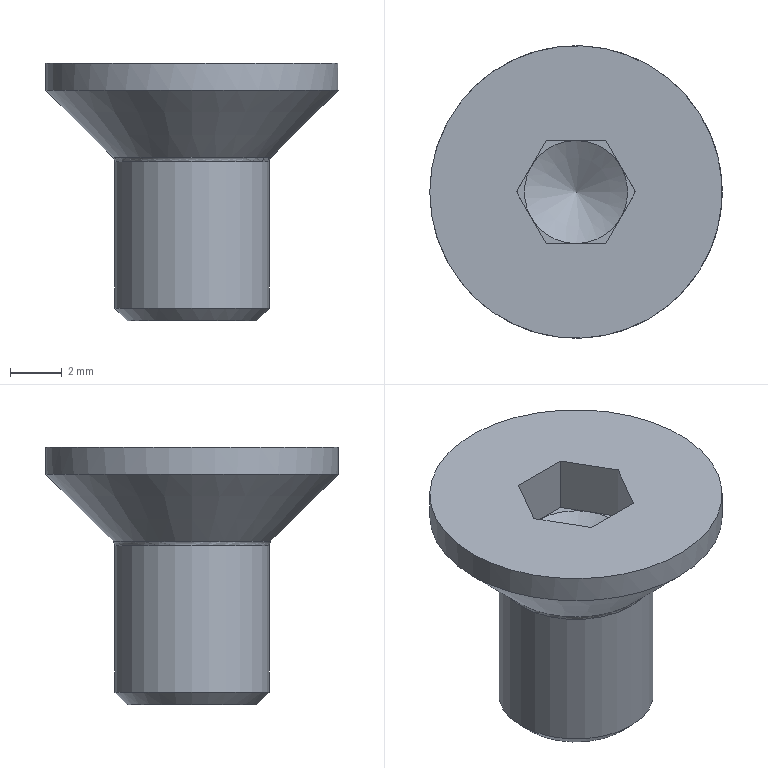Part | STEP file | 冲床-300配套压波_id166_x_t | 1 solid | 20 faces | box 11.34 x 11.34 x 10 mm | volume 408.507 mm3 | plane 14 | cone 3 | cylinder 2 | torus 1 | commonest cylinder face diameters 6 x1 11.34 x1
STEP:
#1=CARTESIAN_POINT('',(1844.33,-85.,217.));
#2=VERTEX_POINT('',#1);
#3=CARTESIAN_POINT('',(1850.,-85.,217.));
#4=DIRECTION('',(0.,0.,-1.));
#5=DIRECTION('',(-1.,0.,0.));
#6=AXIS2_PLACEMENT_3D('',#3,#4,#5);
#7=CIRCLE('',#6,5.67);
#8=EDGE_CURVE('',#2,#2,#7,.T.);
#9=ORIENTED_EDGE('',*,*,#8,.F.);
#10=EDGE_LOOP('',(#9));
#11=FACE_BOUND('',#10,.T.);
#12=CARTESIAN_POINT('',(1847.691,-85.,217.));
#13=VERTEX_POINT('',#12);
#14=CARTESIAN_POINT('',(1848.845,-87.,217.));
#15=VERTEX_POINT('',#14);
#16=CARTESIAN_POINT('',(1847.691,-85.,217.));
#17=DIRECTION('',(0.5,-0.866,0.));
#18=VECTOR('',#17,1.);
#19=LINE('',#16,#18);
#20=EDGE_CURVE('',#13,#15,#19,.T.);
#21=ORIENTED_EDGE('',*,*,#20,.F.);
#22=CARTESIAN_POINT('',(1848.845,-83.,217.));
#23=VERTEX_POINT('',#22);
#24=CARTESIAN_POINT('',(1848.845,-83.,217.));
#25=DIRECTION('',(-0.5,-0.866,0.));
#26=VECTOR('',#25,1.);
#27=LINE('',#24,#26);
#28=EDGE_CURVE('',#23,#13,#27,.T.);
#29=ORIENTED_EDGE('',*,*,#28,.F.);
#30=CARTESIAN_POINT('',(1851.155,-83.,217.));
#31=VERTEX_POINT('',#30);
#32=CARTESIAN_POINT('',(1851.155,-83.,217.));
#33=DIRECTION('',(-1.,0.,0.));
#34=VECTOR('',#33,1.);
#35=LINE('',#32,#34);
#36=EDGE_CURVE('',#31,#23,#35,.T.);
#37=ORIENTED_EDGE('',*,*,#36,.F.);
#38=CARTESIAN_POINT('',(1852.309,-85.,217.));
#39=VERTEX_POINT('',#38);
#40=CARTESIAN_POINT('',(1852.309,-85.,217.));
#41=DIRECTION('',(-0.5,0.866,0.));
#42=VECTOR('',#41,1.);
#43=LINE('',#40,#42);
#44=EDGE_CURVE('',#39,#31,#43,.T.);
#45=ORIENTED_EDGE('',*,*,#44,.F.);
#46=CARTESIAN_POINT('',(1851.155,-87.,217.));
#47=VERTEX_POINT('',#46);
#48=CARTESIAN_POINT('',(1851.155,-87.,217.));
#49=DIRECTION('',(0.5,0.866,0.));
#50=VECTOR('',#49,1.);
#51=LINE('',#48,#50);
#52=EDGE_CURVE('',#47,#39,#51,.T.);
#53=ORIENTED_EDGE('',*,*,#52,.F.);
#54=CARTESIAN_POINT('',(1848.845,-87.,217.));
#55=DIRECTION('',(1.,0.,0.));
#56=VECTOR('',#55,1.);
#57=LINE('',#54,#56);
#58=EDGE_CURVE('',#15,#47,#57,.T.);
#59=ORIENTED_EDGE('',*,*,#58,.F.);
#60=EDGE_LOOP('',(#21,#29,#37,#45,#53,#59));
#61=FACE_BOUND('',#60,.T.);
#62=CARTESIAN_POINT('',(1850.,-85.,217.));
#63=DIRECTION('',(0.,0.,-1.));
#64=DIRECTION('',(-1.,0.,0.));
#65=AXIS2_PLACEMENT_3D('',#62,#63,#64);
#66=PLANE('',#65);
#67=ADVANCED_FACE('',(#11,#61),#66,.F.);
#68=CARTESIAN_POINT('',(1844.33,-85.,215.95));
#69=VERTEX_POINT('',#68);
#70=CARTESIAN_POINT('',(1850.,-85.,215.95));
#71=DIRECTION('',(0.,0.,-1.));
#72=DIRECTION('',(-1.,0.,0.));
#73=AXIS2_PLACEMENT_3D('',#70,#71,#72);
#74=CIRCLE('',#73,5.67);
#75=EDGE_CURVE('',#69,#69,#74,.T.);
#76=ORIENTED_EDGE('',*,*,#75,.F.);
#77=EDGE_LOOP('',(#76));
#78=FACE_BOUND('',#77,.T.);
#79=ORIENTED_EDGE('',*,*,#8,.T.);
#80=EDGE_LOOP('',(#79));
#81=FACE_BOUND('',#80,.T.);
#82=CARTESIAN_POINT('',(1850.,-85.,217.));
#83=DIRECTION('',(0.,0.,-1.));
#84=DIRECTION('',(-1.,0.,0.));
#85=AXIS2_PLACEMENT_3D('',#82,#83,#84);
#86=CYLINDRICAL_SURFACE('',#85,5.67);
#87=ADVANCED_FACE('',(#78,#81),#86,.T.);
#88=CARTESIAN_POINT('',(1853.073,-85.,213.353));
#89=VERTEX_POINT('',#88);
#90=CARTESIAN_POINT('',(1850.,-85.,213.353));
#91=DIRECTION('',(0.,0.,1.));
#92=DIRECTION('',(1.,0.,0.));
#93=AXIS2_PLACEMENT_3D('',#90,#91,#92);
#94=CIRCLE('',#93,3.073);
#95=EDGE_CURVE('',#89,#89,#94,.T.);
#96=ORIENTED_EDGE('',*,*,#95,.T.);
#97=EDGE_LOOP('',(#96));
#98=FACE_BOUND('',#97,.T.);
#99=ORIENTED_EDGE('',*,*,#75,.T.);
#100=EDGE_LOOP('',(#99));
#101=FACE_BOUND('',#100,.T.);
#102=CARTESIAN_POINT('',(1850.,-85.,215.95));
#103=DIRECTION('',(0.,0.,1.));
#104=DIRECTION('',(1.,0.,0.));
#105=AXIS2_PLACEMENT_3D('',#102,#103,#104);
#106=CONICAL_SURFACE('',#105,5.67,45.);
#107=ADVANCED_FACE('',(#98,#101),#106,.T.);
#108=CARTESIAN_POINT('',(1847.,-85.,213.176));
#109=VERTEX_POINT('',#108);
#110=CARTESIAN_POINT('',(1850.,-85.,213.176));
#111=DIRECTION('',(0.,0.,-1.));
#112=DIRECTION('',(-1.,0.,0.));
#113=AXIS2_PLACEMENT_3D('',#110,#111,#112);
#114=CIRCLE('',#113,3.);
#115=EDGE_CURVE('',#109,#109,#114,.T.);
#116=ORIENTED_EDGE('',*,*,#115,.T.);
#117=EDGE_LOOP('',(#116));
#118=FACE_BOUND('',#117,.T.);
#119=CARTESIAN_POINT('',(1853.,-85.,207.5));
#120=VERTEX_POINT('',#119);
#121=CARTESIAN_POINT('',(1850.,-85.,207.5));
#122=DIRECTION('',(0.,0.,1.));
#123=DIRECTION('',(1.,0.,0.));
#124=AXIS2_PLACEMENT_3D('',#121,#122,#123);
#125=CIRCLE('',#124,3.);
#126=EDGE_CURVE('',#120,#120,#125,.T.);
#127=ORIENTED_EDGE('',*,*,#126,.T.);
#128=EDGE_LOOP('',(#127));
#129=FACE_BOUND('',#128,.T.);
#130=CARTESIAN_POINT('',(1850.,-85.,217.));
#131=DIRECTION('',(0.,0.,-1.));
#132=DIRECTION('',(-1.,0.,0.));
#133=AXIS2_PLACEMENT_3D('',#130,#131,#132);
#134=CYLINDRICAL_SURFACE('',#133,3.);
#135=ADVANCED_FACE('',(#118,#129),#134,.T.);
#136=CARTESIAN_POINT('',(1852.5,-85.,207.));
#137=VERTEX_POINT('',#136);
#138=CARTESIAN_POINT('',(1850.,-85.,207.));
#139=DIRECTION('',(0.,0.,-1.));
#140=DIRECTION('',(1.,0.,0.));
#141=AXIS2_PLACEMENT_3D('',#138,#139,#140);
#142=CIRCLE('',#141,2.5);
#143=EDGE_CURVE('',#137,#137,#142,.T.);
#144=ORIENTED_EDGE('',*,*,#143,.T.);
#145=EDGE_LOOP('',(#144));
#146=FACE_OUTER_BOUND('',#145,.T.);
#147=CARTESIAN_POINT('',(1847.,-85.,207.));
#148=DIRECTION('',(0.,0.,1.));
#149=DIRECTION('',(1.,0.,0.));
#150=AXIS2_PLACEMENT_3D('',#147,#148,#149);
#151=PLANE('',#150);
#152=ADVANCED_FACE('',(#146),#151,.F.);
#153=CARTESIAN_POINT('',(1848.268,-86.,214.8));
#154=VERTEX_POINT('',#153);
#155=CARTESIAN_POINT('',(1847.691,-85.,214.8));
#156=VERTEX_POINT('',#155);
#157=CARTESIAN_POINT('',(1847.691,-85.,214.8));
#158=DIRECTION('',(-0.5,0.866,0.));
#159=VECTOR('',#158,1.);
#160=LINE('',#157,#159);
#161=EDGE_CURVE('',#154,#156,#160,.T.);
#162=ORIENTED_EDGE('',*,*,#161,.T.);
#163=CARTESIAN_POINT('',(1847.691,-85.,214.8));
#164=DIRECTION('',(0.,0.,-1.));
#165=VECTOR('',#164,1.);
#166=LINE('',#163,#165);
#167=EDGE_CURVE('',#13,#156,#166,.T.);
#168=ORIENTED_EDGE('',*,*,#167,.F.);
#169=ORIENTED_EDGE('',*,*,#20,.T.);
#170=CARTESIAN_POINT('',(1848.845,-87.,214.8));
#171=VERTEX_POINT('',#170);
#172=CARTESIAN_POINT('',(1848.845,-87.,214.8));
#173=DIRECTION('',(0.,0.,-1.));
#174=VECTOR('',#173,1.);
#175=LINE('',#172,#174);
#176=EDGE_CURVE('',#15,#171,#175,.T.);
#177=ORIENTED_EDGE('',*,*,#176,.T.);
#178=CARTESIAN_POINT('',(1847.691,-85.,214.8));
#179=DIRECTION('',(-0.5,0.866,0.));
#180=VECTOR('',#179,1.);
#181=LINE('',#178,#180);
#182=EDGE_CURVE('',#171,#154,#181,.T.);
#183=ORIENTED_EDGE('',*,*,#182,.T.);
#184=EDGE_LOOP('',(#162,#168,#169,#177,#183));
#185=FACE_OUTER_BOUND('',#184,.T.);
#186=CARTESIAN_POINT('',(1847.691,-85.,214.8));
#187=DIRECTION('',(-0.866,-0.5,0.));
#188=DIRECTION('',(0.5,-0.866,0.));
#189=AXIS2_PLACEMENT_3D('',#186,#187,#188);
#190=PLANE('',#189);
#191=ADVANCED_FACE('',(#185),#190,.F.);
#192=CARTESIAN_POINT('',(1850.,-87.,214.8));
#193=VERTEX_POINT('',#192);
#194=CARTESIAN_POINT('',(1848.845,-87.,214.8));
#195=DIRECTION('',(-1.,0.,0.));
#196=VECTOR('',#195,1.);
#197=LINE('',#194,#196);
#198=EDGE_CURVE('',#193,#171,#197,.T.);
#199=ORIENTED_EDGE('',*,*,#198,.T.);
#200=ORIENTED_EDGE('',*,*,#176,.F.);
#201=ORIENTED_EDGE('',*,*,#58,.T.);
#202=CARTESIAN_POINT('',(1851.155,-87.,214.8));
#203=VERTEX_POINT('',#202);
#204=CARTESIAN_POINT('',(1851.155,-87.,214.8));
#205=DIRECTION('',(0.,0.,-1.));
#206=VECTOR('',#205,1.);
#207=LINE('',#204,#206);
#208=EDGE_CURVE('',#47,#203,#207,.T.);
#209=ORIENTED_EDGE('',*,*,#208,.T.);
#210=CARTESIAN_POINT('',(1848.845,-87.,214.8));
#211=DIRECTION('',(-1.,0.,0.));
#212=VECTOR('',#211,1.);
#213=LINE('',#210,#212);
#214=EDGE_CURVE('',#203,#193,#213,.T.);
#215=ORIENTED_EDGE('',*,*,#214,.T.);
#216=EDGE_LOOP('',(#199,#200,#201,#209,#215));
#217=FACE_OUTER_BOUND('',#216,.T.);
#218=CARTESIAN_POINT('',(1848.845,-87.,214.8));
#219=DIRECTION('',(0.,-1.,0.));
#220=DIRECTION('',(0.,0.,-1.));
#221=AXIS2_PLACEMENT_3D('',#218,#219,#220);
#222=PLANE('',#221);
#223=ADVANCED_FACE('',(#217),#222,.F.);
#224=CARTESIAN_POINT('',(1851.732,-86.,214.8));
#225=VERTEX_POINT('',#224);
#226=CARTESIAN_POINT('',(1851.155,-87.,214.8));
#227=DIRECTION('',(-0.5,-0.866,0.));
#228=VECTOR('',#227,1.);
#229=LINE('',#226,#228);
#230=EDGE_CURVE('',#225,#203,#229,.T.);
#231=ORIENTED_EDGE('',*,*,#230,.T.);
#232=ORIENTED_EDGE('',*,*,#208,.F.);
#233=ORIENTED_EDGE('',*,*,#52,.T.);
#234=CARTESIAN_POINT('',(1852.309,-85.,214.8));
#235=VERTEX_POINT('',#234);
#236=CARTESIAN_POINT('',(1852.309,-85.,214.8));
#237=DIRECTION('',(0.,0.,-1.));
#238=VECTOR('',#237,1.);
#239=LINE('',#236,#238);
#240=EDGE_CURVE('',#39,#235,#239,.T.);
#241=ORIENTED_EDGE('',*,*,#240,.T.);
#242=CARTESIAN_POINT('',(1851.155,-87.,214.8));
#243=DIRECTION('',(-0.5,-0.866,0.));
#244=VECTOR('',#243,1.);
#245=LINE('',#242,#244);
#246=EDGE_CURVE('',#235,#225,#245,.T.);
#247=ORIENTED_EDGE('',*,*,#246,.T.);
#248=EDGE_LOOP('',(#231,#232,#233,#241,#247));
#249=FACE_OUTER_BOUND('',#248,.T.);
#250=CARTESIAN_POINT('',(1851.155,-87.,214.8));
#251=DIRECTION('',(0.866,-0.5,0.));
#252=DIRECTION('',(0.5,0.866,0.));
#253=AXIS2_PLACEMENT_3D('',#250,#251,#252);
#254=PLANE('',#253);
#255=ADVANCED_FACE('',(#249),#254,.F.);
#256=CARTESIAN_POINT('',(1851.732,-84.,214.8));
#257=VERTEX_POINT('',#256);
#258=CARTESIAN_POINT('',(1852.309,-85.,214.8));
#259=DIRECTION('',(0.5,-0.866,0.));
#260=VECTOR('',#259,1.);
#261=LINE('',#258,#260);
#262=EDGE_CURVE('',#257,#235,#261,.T.);
#263=ORIENTED_EDGE('',*,*,#262,.T.);
#264=ORIENTED_EDGE('',*,*,#240,.F.);
#265=ORIENTED_EDGE('',*,*,#44,.T.);
#266=CARTESIAN_POINT('',(1851.155,-83.,214.8));
#267=VERTEX_POINT('',#266);
#268=CARTESIAN_POINT('',(1851.155,-83.,214.8));
#269=DIRECTION('',(0.,0.,-1.));
#270=VECTOR('',#269,1.);
#271=LINE('',#268,#270);
#272=EDGE_CURVE('',#31,#267,#271,.T.);
#273=ORIENTED_EDGE('',*,*,#272,.T.);
#274=CARTESIAN_POINT('',(1852.309,-85.,214.8));
#275=DIRECTION('',(0.5,-0.866,0.));
#276=VECTOR('',#275,1.);
#277=LINE('',#274,#276);
#278=EDGE_CURVE('',#267,#257,#277,.T.);
#279=ORIENTED_EDGE('',*,*,#278,.T.);
#280=EDGE_LOOP('',(#263,#264,#265,#273,#279));
#281=FACE_OUTER_BOUND('',#280,.T.);
#282=CARTESIAN_POINT('',(1852.309,-85.,214.8));
#283=DIRECTION('',(0.866,0.5,0.));
#284=DIRECTION('',(-0.5,0.866,0.));
#285=AXIS2_PLACEMENT_3D('',#282,#283,#284);
#286=PLANE('',#285);
#287=ADVANCED_FACE('',(#281),#286,.F.);
#288=CARTESIAN_POINT('',(1850.,-83.,214.8));
#289=VERTEX_POINT('',#288);
#290=CARTESIAN_POINT('',(1851.155,-83.,214.8));
#291=DIRECTION('',(1.,0.,0.));
#292=VECTOR('',#291,1.);
#293=LINE('',#290,#292);
#294=EDGE_CURVE('',#289,#267,#293,.T.);
#295=ORIENTED_EDGE('',*,*,#294,.T.);
#296=ORIENTED_EDGE('',*,*,#272,.F.);
#297=ORIENTED_EDGE('',*,*,#36,.T.);
#298=CARTESIAN_POINT('',(1848.845,-83.,214.8));
#299=VERTEX_POINT('',#298);
#300=CARTESIAN_POINT('',(1848.845,-83.,214.8));
#301=DIRECTION('',(0.,0.,-1.));
#302=VECTOR('',#301,1.);
#303=LINE('',#300,#302);
#304=EDGE_CURVE('',#23,#299,#303,.T.);
#305=ORIENTED_EDGE('',*,*,#304,.T.);
#306=CARTESIAN_POINT('',(1851.155,-83.,214.8));
#307=DIRECTION('',(1.,0.,0.));
#308=VECTOR('',#307,1.);
#309=LINE('',#306,#308);
#310=EDGE_CURVE('',#299,#289,#309,.T.);
#311=ORIENTED_EDGE('',*,*,#310,.T.);
#312=EDGE_LOOP('',(#295,#296,#297,#305,#311));
#313=FACE_OUTER_BOUND('',#312,.T.);
#314=CARTESIAN_POINT('',(1851.155,-83.,214.8));
#315=DIRECTION('',(0.,1.,0.));
#316=DIRECTION('',(-1.,0.,0.));
#317=AXIS2_PLACEMENT_3D('',#314,#315,#316);
#318=PLANE('',#317);
#319=ADVANCED_FACE('',(#313),#318,.F.);
#320=CARTESIAN_POINT('',(1848.268,-84.,214.8));
#321=VERTEX_POINT('',#320);
#322=CARTESIAN_POINT('',(1848.845,-83.,214.8));
#323=DIRECTION('',(0.5,0.866,0.));
#324=VECTOR('',#323,1.);
#325=LINE('',#322,#324);
#326=EDGE_CURVE('',#321,#299,#325,.T.);
#327=ORIENTED_EDGE('',*,*,#326,.T.);
#328=ORIENTED_EDGE('',*,*,#304,.F.);
#329=ORIENTED_EDGE('',*,*,#28,.T.);
#330=ORIENTED_EDGE('',*,*,#167,.T.);
#331=CARTESIAN_POINT('',(1848.845,-83.,214.8));
#332=DIRECTION('',(0.5,0.866,0.));
#333=VECTOR('',#332,1.);
#334=LINE('',#331,#333);
#335=EDGE_CURVE('',#156,#321,#334,.T.);
#336=ORIENTED_EDGE('',*,*,#335,.T.);
#337=EDGE_LOOP('',(#327,#328,#329,#330,#336));
#338=FACE_OUTER_BOUND('',#337,.T.);
#339=CARTESIAN_POINT('',(1848.845,-83.,214.8));
#340=DIRECTION('',(-0.866,0.5,0.));
#341=DIRECTION('',(-0.5,-0.866,0.));
#342=AXIS2_PLACEMENT_3D('',#339,#340,#341);
#343=PLANE('',#342);
#344=ADVANCED_FACE('',(#338),#343,.F.);
#345=CARTESIAN_POINT('',(1850.,-85.,214.8));
#346=DIRECTION('',(0.,0.,1.));
#347=DIRECTION('',(-1.,0.,0.));
#348=AXIS2_PLACEMENT_3D('',#345,#346,#347);
#349=CIRCLE('',#348,2.);
#350=EDGE_CURVE('',#193,#225,#349,.T.);
#351=ORIENTED_EDGE('',*,*,#350,.F.);
#352=ORIENTED_EDGE('',*,*,#214,.F.);
#353=ORIENTED_EDGE('',*,*,#230,.F.);
#354=EDGE_LOOP('',(#351,#352,#353));
#355=FACE_OUTER_BOUND('',#354,.T.);
#356=CARTESIAN_POINT('',(1850.,-85.,214.8));
#357=DIRECTION('',(0.,0.,1.));
#358=DIRECTION('',(1.,0.,0.));
#359=AXIS2_PLACEMENT_3D('',#356,#357,#358);
#360=PLANE('',#359);
#361=ADVANCED_FACE('',(#355),#360,.T.);
#362=CARTESIAN_POINT('',(1850.,-85.,214.8));
#363=DIRECTION('',(0.,0.,1.));
#364=DIRECTION('',(-1.,0.,0.));
#365=AXIS2_PLACEMENT_3D('',#362,#363,#364);
#366=CIRCLE('',#365,2.);
#367=EDGE_CURVE('',#154,#193,#366,.T.);
#368=ORIENTED_EDGE('',*,*,#367,.F.);
#369=ORIENTED_EDGE('',*,*,#182,.F.);
#370=ORIENTED_EDGE('',*,*,#198,.F.);
#371=EDGE_LOOP('',(#368,#369,#370));
#372=FACE_OUTER_BOUND('',#371,.T.);
#373=CARTESIAN_POINT('',(1850.,-85.,214.8));
#374=DIRECTION('',(0.,0.,1.));
#375=DIRECTION('',(1.,0.,0.));
#376=AXIS2_PLACEMENT_3D('',#373,#374,#375);
#377=PLANE('',#376);
#378=ADVANCED_FACE('',(#372),#377,.T.);
#379=CARTESIAN_POINT('',(1850.,-85.,214.8));
#380=DIRECTION('',(0.,0.,1.));
#381=DIRECTION('',(-1.,0.,0.));
#382=AXIS2_PLACEMENT_3D('',#379,#380,#381);
#383=CIRCLE('',#382,2.);
#384=EDGE_CURVE('',#321,#154,#383,.T.);
#385=ORIENTED_EDGE('',*,*,#384,.F.);
#386=ORIENTED_EDGE('',*,*,#335,.F.);
#387=ORIENTED_EDGE('',*,*,#161,.F.);
#388=EDGE_LOOP('',(#385,#386,#387));
#389=FACE_OUTER_BOUND('',#388,.T.);
#390=CARTESIAN_POINT('',(1850.,-85.,214.8));
#391=DIRECTION('',(0.,0.,1.));
#392=DIRECTION('',(1.,0.,0.));
#393=AXIS2_PLACEMENT_3D('',#390,#391,#392);
#394=PLANE('',#393);
#395=ADVANCED_FACE('',(#389),#394,.T.);
#396=CARTESIAN_POINT('',(1850.,-85.,214.8));
#397=DIRECTION('',(0.,0.,1.));
#398=DIRECTION('',(-1.,0.,0.));
#399=AXIS2_PLACEMENT_3D('',#396,#397,#398);
#400=CIRCLE('',#399,2.);
#401=EDGE_CURVE('',#289,#321,#400,.T.);
#402=ORIENTED_EDGE('',*,*,#401,.F.);
#403=ORIENTED_EDGE('',*,*,#310,.F.);
#404=ORIENTED_EDGE('',*,*,#326,.F.);
#405=EDGE_LOOP('',(#402,#403,#404));
#406=FACE_OUTER_BOUND('',#405,.T.);
#407=CARTESIAN_POINT('',(1850.,-85.,214.8));
#408=DIRECTION('',(0.,0.,1.));
#409=DIRECTION('',(1.,0.,0.));
#410=AXIS2_PLACEMENT_3D('',#407,#408,#409);
#411=PLANE('',#410);
#412=ADVANCED_FACE('',(#406),#411,.T.);
#413=CARTESIAN_POINT('',(1850.,-85.,214.8));
#414=DIRECTION('',(0.,0.,1.));
#415=DIRECTION('',(-1.,0.,0.));
#416=AXIS2_PLACEMENT_3D('',#413,#414,#415);
#417=CIRCLE('',#416,2.);
#418=EDGE_CURVE('',#257,#289,#417,.T.);
#419=ORIENTED_EDGE('',*,*,#418,.F.);
#420=ORIENTED_EDGE('',*,*,#278,.F.);
#421=ORIENTED_EDGE('',*,*,#294,.F.);
#422=EDGE_LOOP('',(#419,#420,#421));
#423=FACE_OUTER_BOUND('',#422,.T.);
#424=CARTESIAN_POINT('',(1850.,-85.,214.8));
#425=DIRECTION('',(0.,0.,1.));
#426=DIRECTION('',(1.,0.,0.));
#427=AXIS2_PLACEMENT_3D('',#424,#425,#426);
#428=PLANE('',#427);
#429=ADVANCED_FACE('',(#423),#428,.T.);
#430=CARTESIAN_POINT('',(1850.,-85.,214.8));
#431=DIRECTION('',(0.,0.,1.));
#432=DIRECTION('',(-1.,0.,0.));
#433=AXIS2_PLACEMENT_3D('',#430,#431,#432);
#434=CIRCLE('',#433,2.);
#435=EDGE_CURVE('',#225,#257,#434,.T.);
#436=ORIENTED_EDGE('',*,*,#435,.F.);
#437=ORIENTED_EDGE('',*,*,#246,.F.);
#438=ORIENTED_EDGE('',*,*,#262,.F.);
#439=EDGE_LOOP('',(#436,#437,#438));
#440=FACE_OUTER_BOUND('',#439,.T.);
#441=CARTESIAN_POINT('',(1850.,-85.,214.8));
#442=DIRECTION('',(0.,0.,1.));
#443=DIRECTION('',(1.,0.,0.));
#444=AXIS2_PLACEMENT_3D('',#441,#442,#443);
#445=PLANE('',#444);
#446=ADVANCED_FACE('',(#440),#445,.T.);
#447=ORIENTED_EDGE('',*,*,#367,.T.);
#448=ORIENTED_EDGE('',*,*,#350,.T.);
#449=ORIENTED_EDGE('',*,*,#435,.T.);
#450=ORIENTED_EDGE('',*,*,#418,.T.);
#451=ORIENTED_EDGE('',*,*,#401,.T.);
#452=ORIENTED_EDGE('',*,*,#384,.T.);
#453=EDGE_LOOP('',(#447,#448,#449,#450,#451,#452));
#454=FACE_BOUND('',#453,.T.);
#455=CARTESIAN_POINT('',(1850.,-85.,213.598));
#456=VERTEX_POINT('',#455);
#457=VERTEX_LOOP('',#456);
#458=FACE_BOUND('',#457,.T.);
#459=CARTESIAN_POINT('',(1850.,-85.,214.8));
#460=DIRECTION('',(0.,0.,1.));
#461=DIRECTION('',(1.,0.,0.));
#462=AXIS2_PLACEMENT_3D('',#459,#460,#461);
#463=CONICAL_SURFACE('',#462,2.,59.);
#464=ADVANCED_FACE('',(#454,#458),#463,.F.);
#465=ORIENTED_EDGE('',*,*,#126,.F.);
#466=EDGE_LOOP('',(#465));
#467=FACE_BOUND('',#466,.T.);
#468=ORIENTED_EDGE('',*,*,#143,.F.);
#469=EDGE_LOOP('',(#468));
#470=FACE_BOUND('',#469,.T.);
#471=CARTESIAN_POINT('',(1850.,-85.,207.));
#472=DIRECTION('',(0.,0.,1.));
#473=DIRECTION('',(1.,0.,0.));
#474=AXIS2_PLACEMENT_3D('',#471,#472,#473);
#475=CONICAL_SURFACE('',#474,2.5,45.);
#476=ADVANCED_FACE('',(#467,#470),#475,.T.);
#477=ORIENTED_EDGE('',*,*,#95,.F.);
#478=EDGE_LOOP('',(#477));
#479=FACE_BOUND('',#478,.T.);
#480=ORIENTED_EDGE('',*,*,#115,.F.);
#481=EDGE_LOOP('',(#480));
#482=FACE_BOUND('',#481,.T.);
#483=CARTESIAN_POINT('',(1850.,-85.,213.176));
#484=DIRECTION('',(0.,0.,-1.));
#485=DIRECTION('',(-1.,0.,0.));
#486=AXIS2_PLACEMENT_3D('',#483,#484,#485);
#487=TOROIDAL_SURFACE('',#486,3.25,0.25);
#488=ADVANCED_FACE('',(#479,#482),#487,.F.);
#489=CLOSED_SHELL('',(#67,#87,#107,#135,#152,#191,#223,#255,#287,#319,#344,#361,#378,#395,#412,#429,#446,#464,#476,#488));
#490=MANIFOLD_SOLID_BREP('',#489);
#491=(LENGTH_UNIT()NAMED_UNIT(*)SI_UNIT(.MILLI.,.METRE.));
#492=UNCERTAINTY_MEASURE_WITH_UNIT(LENGTH_MEASURE(0.00002),#491,'','');
#493=(NAMED_UNIT(*)PLANE_ANGLE_UNIT()SI_UNIT($,.RADIAN.));
#494=PLANE_ANGLE_MEASURE_WITH_UNIT(PLANE_ANGLE_MEASURE(0.01745),#493);
#495=DIMENSIONAL_EXPONENTS(0.,0.,0.,0.,0.,0.,0.);
#496=(CONVERSION_BASED_UNIT('DEGREE',#494)NAMED_UNIT(#495)PLANE_ANGLE_UNIT());
#497=(NAMED_UNIT(*)SI_UNIT($,.STERADIAN.)SOLID_ANGLE_UNIT());
#498=(GEOMETRIC_REPRESENTATION_CONTEXT(3)GLOBAL_UNCERTAINTY_ASSIGNED_CONTEXT((#492))GLOBAL_UNIT_ASSIGNED_CONTEXT((#491,#496,#497))REPRESENTATION_CONTEXT('',''));
#499=ADVANCED_BREP_SHAPE_REPRESENTATION('',(#490),#498);